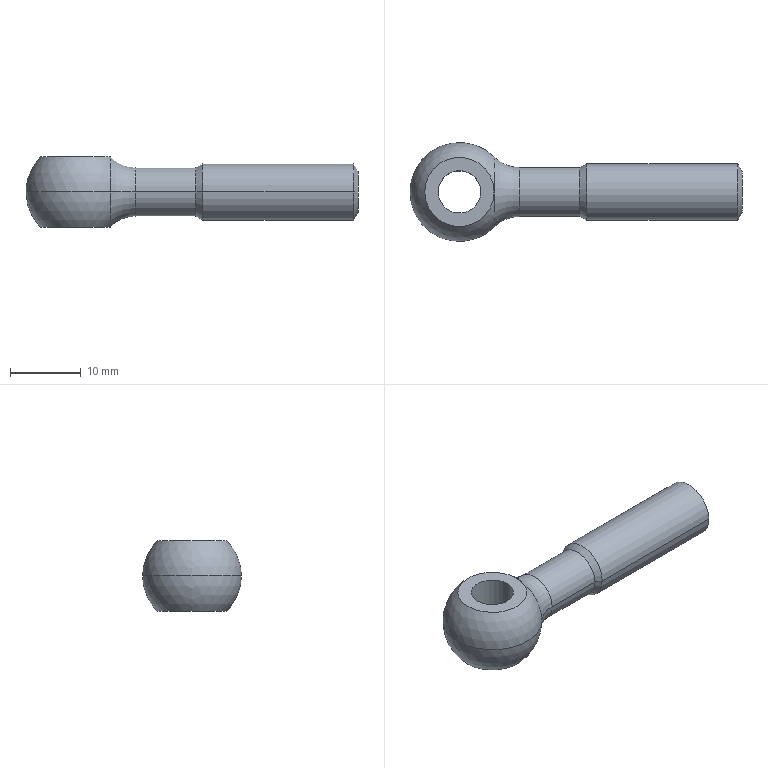Part | SolidWorks | features Cut 2, Revolution 2, Chamfer 1, Fillet 1, LPattern 1, RevCut 1 | 1 solid | 17 faces | box 47 x 14 x 10 mm | volume 2546 mm3 | cylinder 6 | cone 4 | plane 3 | torus 2 | sphere 2 | commonest cylinder face diameters 6 x2 6.918 x2 8 x2
STEP:
#1=CARTESIAN_POINT('',(4.965,4.934,0.));
#2=VERTEX_POINT('',#1);
#3=CARTESIAN_POINT('',(4.965,-4.934,0.));
#4=VERTEX_POINT('',#3);
#5=CARTESIAN_POINT('',(4.965,0.,0.));
#6=DIRECTION('',(-1.,0.,0.));
#7=DIRECTION('',(0.,-1.,0.));
#8=AXIS2_PLACEMENT_3D('',#5,#6,#7);
#9=CIRCLE('',#8,4.934);
#10=EDGE_CURVE('',#2,#4,#9,.T.);
#11=ORIENTED_EDGE('',*,*,#10,.F.);
#12=CARTESIAN_POINT('',(8.512,3.459,0.));
#13=VERTEX_POINT('',#12);
#14=CARTESIAN_POINT('',(8.512,8.459,0.));
#15=DIRECTION('',(0.,0.,1.));
#16=DIRECTION('',(0.,-1.,0.));
#17=AXIS2_PLACEMENT_3D('',#14,#15,#16);
#18=CIRCLE('',#17,5.);
#19=EDGE_CURVE('',#2,#13,#18,.T.);
#20=ORIENTED_EDGE('',*,*,#19,.T.);
#21=CARTESIAN_POINT('',(8.512,-3.459,0.));
#22=VERTEX_POINT('',#21);
#23=CARTESIAN_POINT('',(8.512,0.,0.));
#24=DIRECTION('',(1.,0.,0.));
#25=DIRECTION('',(0.,-1.,0.));
#26=AXIS2_PLACEMENT_3D('',#23,#24,#25);
#27=CIRCLE('',#26,3.459);
#28=EDGE_CURVE('',#22,#13,#27,.T.);
#29=ORIENTED_EDGE('',*,*,#28,.F.);
#30=CARTESIAN_POINT('',(8.512,-8.459,0.));
#31=DIRECTION('',(0.,0.,-1.));
#32=DIRECTION('',(0.,1.,0.));
#33=AXIS2_PLACEMENT_3D('',#30,#31,#32);
#34=CIRCLE('',#33,5.);
#35=EDGE_CURVE('',#4,#22,#34,.T.);
#36=ORIENTED_EDGE('',*,*,#35,.F.);
#37=EDGE_LOOP('',(#11,#20,#29,#36));
#38=FACE_OUTER_BOUND('',#37,.T.);
#39=CARTESIAN_POINT('',(8.512,0.,0.));
#40=DIRECTION('',(-1.,0.,0.));
#41=DIRECTION('',(0.,-1.,0.));
#42=AXIS2_PLACEMENT_3D('',#39,#40,#41);
#43=TOROIDAL_SURFACE('',#42,8.459,5.);
#44=ADVANCED_FACE('',(#38),#43,.F.);
#45=CARTESIAN_POINT('',(40.,-2.918,0.));
#46=VERTEX_POINT('',#45);
#47=CARTESIAN_POINT('',(40.,2.917,0.));
#48=VERTEX_POINT('',#47);
#49=CARTESIAN_POINT('',(40.,0.,0.));
#50=DIRECTION('',(-1.,0.,0.));
#51=DIRECTION('',(0.,-1.,0.));
#52=AXIS2_PLACEMENT_3D('',#49,#50,#51);
#53=CIRCLE('',#52,2.918);
#54=EDGE_CURVE('',#46,#48,#53,.T.);
#55=ORIENTED_EDGE('',*,*,#54,.T.);
#56=CARTESIAN_POINT('',(39.375,4.,0.));
#57=VERTEX_POINT('',#56);
#58=CARTESIAN_POINT('',(39.375,4.,0.));
#59=DIRECTION('',(-0.5,0.866,0.));
#60=VECTOR('',#59,1000.);
#61=LINE('',#58,#60);
#62=EDGE_CURVE('',#48,#57,#61,.T.);
#63=ORIENTED_EDGE('',*,*,#62,.T.);
#64=CARTESIAN_POINT('',(39.375,-4.,0.));
#65=VERTEX_POINT('',#64);
#66=CARTESIAN_POINT('',(39.375,0.,0.));
#67=DIRECTION('',(-1.,0.,0.));
#68=DIRECTION('',(0.,-1.,0.));
#69=AXIS2_PLACEMENT_3D('',#66,#67,#68);
#70=CIRCLE('',#69,4.);
#71=EDGE_CURVE('',#65,#57,#70,.T.);
#72=ORIENTED_EDGE('',*,*,#71,.F.);
#73=CARTESIAN_POINT('',(39.375,-4.,0.));
#74=DIRECTION('',(-0.5,-0.866,0.));
#75=VECTOR('',#74,1000.);
#76=LINE('',#73,#75);
#77=EDGE_CURVE('',#46,#65,#76,.T.);
#78=ORIENTED_EDGE('',*,*,#77,.F.);
#79=EDGE_LOOP('',(#55,#63,#72,#78));
#80=FACE_OUTER_BOUND('',#79,.T.);
#81=CARTESIAN_POINT('',(39.375,0.,0.));
#82=DIRECTION('',(-1.,0.,0.));
#83=DIRECTION('',(0.,-1.,0.));
#84=AXIS2_PLACEMENT_3D('',#81,#82,#83);
#85=CONICAL_SURFACE('',#84,4.,1.047);
#86=ADVANCED_FACE('',(#80),#85,.T.);
#87=CARTESIAN_POINT('',(17.063,-3.459,0.));
#88=VERTEX_POINT('',#87);
#89=CARTESIAN_POINT('',(17.063,3.459,0.));
#90=VERTEX_POINT('',#89);
#91=CARTESIAN_POINT('',(17.063,0.,0.));
#92=DIRECTION('',(-1.,0.,0.));
#93=DIRECTION('',(0.,-1.,0.));
#94=AXIS2_PLACEMENT_3D('',#91,#92,#93);
#95=CIRCLE('',#94,3.459);
#96=EDGE_CURVE('',#88,#90,#95,.T.);
#97=ORIENTED_EDGE('',*,*,#96,.F.);
#98=CARTESIAN_POINT('',(18.,-4.,0.));
#99=VERTEX_POINT('',#98);
#100=CARTESIAN_POINT('',(18.,-4.,0.));
#101=DIRECTION('',(0.866,-0.5,0.));
#102=VECTOR('',#101,1000.);
#103=LINE('',#100,#102);
#104=EDGE_CURVE('',#88,#99,#103,.T.);
#105=ORIENTED_EDGE('',*,*,#104,.T.);
#106=CARTESIAN_POINT('',(18.,4.,0.));
#107=VERTEX_POINT('',#106);
#108=CARTESIAN_POINT('',(18.,0.,0.));
#109=DIRECTION('',(-1.,0.,0.));
#110=DIRECTION('',(0.,-1.,0.));
#111=AXIS2_PLACEMENT_3D('',#108,#109,#110);
#112=CIRCLE('',#111,4.);
#113=EDGE_CURVE('',#99,#107,#112,.T.);
#114=ORIENTED_EDGE('',*,*,#113,.T.);
#115=CARTESIAN_POINT('',(18.,4.,0.));
#116=DIRECTION('',(0.866,0.5,0.));
#117=VECTOR('',#116,1000.);
#118=LINE('',#115,#117);
#119=EDGE_CURVE('',#90,#107,#118,.T.);
#120=ORIENTED_EDGE('',*,*,#119,.F.);
#121=EDGE_LOOP('',(#97,#105,#114,#120));
#122=FACE_OUTER_BOUND('',#121,.T.);
#123=CARTESIAN_POINT('',(18.,0.,0.));
#124=DIRECTION('',(1.,0.,0.));
#125=DIRECTION('',(0.,1.,0.));
#126=AXIS2_PLACEMENT_3D('',#123,#124,#125);
#127=CONICAL_SURFACE('',#126,4.,0.5236);
#128=ADVANCED_FACE('',(#122),#127,.T.);
#129=ORIENTED_EDGE('',*,*,#96,.T.);
#130=CARTESIAN_POINT('',(0.,3.459,0.));
#131=DIRECTION('',(-1.,0.,0.));
#132=VECTOR('',#131,1000.);
#133=LINE('',#130,#132);
#134=EDGE_CURVE('',#90,#13,#133,.T.);
#135=ORIENTED_EDGE('',*,*,#134,.T.);
#136=CARTESIAN_POINT('',(8.512,0.,0.));
#137=DIRECTION('',(1.,0.,0.));
#138=DIRECTION('',(0.,-1.,0.));
#139=AXIS2_PLACEMENT_3D('',#136,#137,#138);
#140=CIRCLE('',#139,3.459);
#141=EDGE_CURVE('',#13,#22,#140,.T.);
#142=ORIENTED_EDGE('',*,*,#141,.T.);
#143=CARTESIAN_POINT('',(0.,-3.459,0.));
#144=DIRECTION('',(-1.,0.,0.));
#145=VECTOR('',#144,1000.);
#146=LINE('',#143,#145);
#147=EDGE_CURVE('',#88,#22,#146,.T.);
#148=ORIENTED_EDGE('',*,*,#147,.F.);
#149=EDGE_LOOP('',(#129,#135,#142,#148));
#150=FACE_OUTER_BOUND('',#149,.T.);
#151=CARTESIAN_POINT('',(0.,0.,0.));
#152=DIRECTION('',(-1.,0.,0.));
#153=DIRECTION('',(0.,-1.,0.));
#154=AXIS2_PLACEMENT_3D('',#151,#152,#153);
#155=CYLINDRICAL_SURFACE('',#154,3.459);
#156=ADVANCED_FACE('',(#150),#155,.T.);
#157=CARTESIAN_POINT('',(-3.,0.,-5.));
#158=VERTEX_POINT('',#157);
#159=CARTESIAN_POINT('',(3.,0.,-5.));
#160=VERTEX_POINT('',#159);
#161=CARTESIAN_POINT('',(0.,0.,-5.));
#162=DIRECTION('',(0.,0.,1.));
#163=DIRECTION('',(1.,0.,0.));
#164=AXIS2_PLACEMENT_3D('',#161,#162,#163);
#165=CIRCLE('',#164,3.);
#166=EDGE_CURVE('',#158,#160,#165,.T.);
#167=ORIENTED_EDGE('',*,*,#166,.F.);
#168=CARTESIAN_POINT('',(-3.,0.,5.));
#169=VERTEX_POINT('',#168);
#170=CARTESIAN_POINT('',(-3.,0.,-5.));
#171=DIRECTION('',(0.,0.,1.));
#172=VECTOR('',#171,1000.);
#173=LINE('',#170,#172);
#174=EDGE_CURVE('',#158,#169,#173,.T.);
#175=ORIENTED_EDGE('',*,*,#174,.T.);
#176=CARTESIAN_POINT('',(3.,0.,5.));
#177=VERTEX_POINT('',#176);
#178=CARTESIAN_POINT('',(0.,0.,5.));
#179=DIRECTION('',(0.,0.,1.));
#180=DIRECTION('',(1.,0.,0.));
#181=AXIS2_PLACEMENT_3D('',#178,#179,#180);
#182=CIRCLE('',#181,3.);
#183=EDGE_CURVE('',#169,#177,#182,.T.);
#184=ORIENTED_EDGE('',*,*,#183,.T.);
#185=CARTESIAN_POINT('',(3.,0.,-5.));
#186=DIRECTION('',(0.,0.,1.));
#187=VECTOR('',#186,1000.);
#188=LINE('',#185,#187);
#189=EDGE_CURVE('',#160,#177,#188,.T.);
#190=ORIENTED_EDGE('',*,*,#189,.F.);
#191=EDGE_LOOP('',(#167,#175,#184,#190));
#192=FACE_OUTER_BOUND('',#191,.T.);
#193=CARTESIAN_POINT('',(0.,0.,-5.));
#194=DIRECTION('',(0.,0.,1.));
#195=DIRECTION('',(1.,0.,0.));
#196=AXIS2_PLACEMENT_3D('',#193,#194,#195);
#197=CYLINDRICAL_SURFACE('',#196,3.);
#198=ADVANCED_FACE('',(#192),#197,.F.);
#199=CARTESIAN_POINT('',(4.899,0.,-5.));
#200=VERTEX_POINT('',#199);
#201=CARTESIAN_POINT('',(-4.899,0.,-5.));
#202=VERTEX_POINT('',#201);
#203=CARTESIAN_POINT('',(0.,0.,-5.));
#204=DIRECTION('',(0.,0.,1.));
#205=DIRECTION('',(1.,0.,0.));
#206=AXIS2_PLACEMENT_3D('',#203,#204,#205);
#207=CIRCLE('',#206,4.899);
#208=EDGE_CURVE('',#200,#202,#207,.T.);
#209=ORIENTED_EDGE('',*,*,#208,.T.);
#210=CARTESIAN_POINT('',(0.,0.,-5.));
#211=DIRECTION('',(0.,0.,1.));
#212=DIRECTION('',(1.,0.,0.));
#213=AXIS2_PLACEMENT_3D('',#210,#211,#212);
#214=CIRCLE('',#213,4.899);
#215=EDGE_CURVE('',#202,#200,#214,.T.);
#216=ORIENTED_EDGE('',*,*,#215,.T.);
#217=EDGE_LOOP('',(#209,#216));
#218=FACE_BOUND('',#217,.T.);
#219=ORIENTED_EDGE('',*,*,#10,.T.);
#220=CARTESIAN_POINT('',(-7.,0.,0.));
#221=VERTEX_POINT('',#220);
#222=CARTESIAN_POINT('',(0.,0.,0.));
#223=DIRECTION('',(0.,0.,-1.));
#224=DIRECTION('',(0.,1.,0.));
#225=AXIS2_PLACEMENT_3D('',#222,#223,#224);
#226=CIRCLE('',#225,7.);
#227=EDGE_CURVE('',#4,#221,#226,.T.);
#228=ORIENTED_EDGE('',*,*,#227,.T.);
#229=CARTESIAN_POINT('',(0.,0.,0.));
#230=DIRECTION('',(0.,0.,1.));
#231=DIRECTION('',(0.,-1.,0.));
#232=AXIS2_PLACEMENT_3D('',#229,#230,#231);
#233=CIRCLE('',#232,7.);
#234=EDGE_CURVE('',#2,#221,#233,.T.);
#235=ORIENTED_EDGE('',*,*,#234,.F.);
#236=EDGE_LOOP('',(#219,#228,#235));
#237=FACE_OUTER_BOUND('',#236,.T.);
#238=CARTESIAN_POINT('',(0.,0.,0.));
#239=DIRECTION('',(0.,0.,-1.));
#240=DIRECTION('',(0.,1.,0.));
#241=AXIS2_PLACEMENT_3D('',#238,#239,#240);
#242=SPHERICAL_SURFACE('',#241,7.);
#243=ADVANCED_FACE('',(#218,#237),#242,.T.);
#244=ORIENTED_EDGE('',*,*,#71,.T.);
#245=CARTESIAN_POINT('',(0.,4.,0.));
#246=DIRECTION('',(-1.,0.,0.));
#247=VECTOR('',#246,1000.);
#248=LINE('',#245,#247);
#249=EDGE_CURVE('',#57,#107,#248,.T.);
#250=ORIENTED_EDGE('',*,*,#249,.T.);
#251=ORIENTED_EDGE('',*,*,#113,.F.);
#252=CARTESIAN_POINT('',(0.,-4.,0.));
#253=DIRECTION('',(-1.,0.,0.));
#254=VECTOR('',#253,1000.);
#255=LINE('',#252,#254);
#256=EDGE_CURVE('',#65,#99,#255,.T.);
#257=ORIENTED_EDGE('',*,*,#256,.F.);
#258=EDGE_LOOP('',(#244,#250,#251,#257));
#259=FACE_OUTER_BOUND('',#258,.T.);
#260=CARTESIAN_POINT('',(0.,0.,0.));
#261=DIRECTION('',(-1.,0.,0.));
#262=DIRECTION('',(0.,-1.,0.));
#263=AXIS2_PLACEMENT_3D('',#260,#261,#262);
#264=CYLINDRICAL_SURFACE('',#263,4.);
#265=ADVANCED_FACE('',(#259),#264,.T.);
#266=ORIENTED_EDGE('',*,*,#249,.F.);
#267=CARTESIAN_POINT('',(39.375,0.,0.));
#268=DIRECTION('',(-1.,0.,0.));
#269=DIRECTION('',(0.,-1.,0.));
#270=AXIS2_PLACEMENT_3D('',#267,#268,#269);
#271=CIRCLE('',#270,4.);
#272=EDGE_CURVE('',#57,#65,#271,.T.);
#273=ORIENTED_EDGE('',*,*,#272,.T.);
#274=ORIENTED_EDGE('',*,*,#256,.T.);
#275=CARTESIAN_POINT('',(18.,0.,0.));
#276=DIRECTION('',(-1.,0.,0.));
#277=DIRECTION('',(0.,-1.,0.));
#278=AXIS2_PLACEMENT_3D('',#275,#276,#277);
#279=CIRCLE('',#278,4.);
#280=EDGE_CURVE('',#107,#99,#279,.T.);
#281=ORIENTED_EDGE('',*,*,#280,.F.);
#282=EDGE_LOOP('',(#266,#273,#274,#281));
#283=FACE_OUTER_BOUND('',#282,.T.);
#284=CARTESIAN_POINT('',(0.,0.,0.));
#285=DIRECTION('',(-1.,0.,0.));
#286=DIRECTION('',(0.,-1.,0.));
#287=AXIS2_PLACEMENT_3D('',#284,#285,#286);
#288=CYLINDRICAL_SURFACE('',#287,4.);
#289=ADVANCED_FACE('',(#283),#288,.T.);
#290=ORIENTED_EDGE('',*,*,#227,.F.);
#291=CARTESIAN_POINT('',(4.965,0.,0.));
#292=DIRECTION('',(-1.,0.,0.));
#293=DIRECTION('',(0.,-1.,0.));
#294=AXIS2_PLACEMENT_3D('',#291,#292,#293);
#295=CIRCLE('',#294,4.934);
#296=EDGE_CURVE('',#4,#2,#295,.T.);
#297=ORIENTED_EDGE('',*,*,#296,.T.);
#298=ORIENTED_EDGE('',*,*,#234,.T.);
#299=EDGE_LOOP('',(#290,#297,#298));
#300=FACE_OUTER_BOUND('',#299,.T.);
#301=CARTESIAN_POINT('',(-4.899,0.,5.));
#302=VERTEX_POINT('',#301);
#303=CARTESIAN_POINT('',(4.899,0.,5.));
#304=VERTEX_POINT('',#303);
#305=CARTESIAN_POINT('',(0.,0.,5.));
#306=DIRECTION('',(0.,0.,-1.));
#307=DIRECTION('',(-1.,0.,0.));
#308=AXIS2_PLACEMENT_3D('',#305,#306,#307);
#309=CIRCLE('',#308,4.899);
#310=EDGE_CURVE('',#302,#304,#309,.T.);
#311=ORIENTED_EDGE('',*,*,#310,.T.);
#312=CARTESIAN_POINT('',(0.,0.,5.));
#313=DIRECTION('',(0.,0.,-1.));
#314=DIRECTION('',(-1.,0.,0.));
#315=AXIS2_PLACEMENT_3D('',#312,#313,#314);
#316=CIRCLE('',#315,4.899);
#317=EDGE_CURVE('',#304,#302,#316,.T.);
#318=ORIENTED_EDGE('',*,*,#317,.T.);
#319=EDGE_LOOP('',(#311,#318));
#320=FACE_BOUND('',#319,.T.);
#321=CARTESIAN_POINT('',(0.,0.,0.));
#322=DIRECTION('',(0.,0.,-1.));
#323=DIRECTION('',(0.,1.,0.));
#324=AXIS2_PLACEMENT_3D('',#321,#322,#323);
#325=SPHERICAL_SURFACE('',#324,7.);
#326=ADVANCED_FACE('',(#300,#320),#325,.T.);
#327=CARTESIAN_POINT('',(0.,0.,5.));
#328=DIRECTION('',(0.,0.,1.));
#329=DIRECTION('',(1.,0.,0.));
#330=AXIS2_PLACEMENT_3D('',#327,#328,#329);
#331=CIRCLE('',#330,3.);
#332=EDGE_CURVE('',#177,#169,#331,.T.);
#333=ORIENTED_EDGE('',*,*,#332,.F.);
#334=ORIENTED_EDGE('',*,*,#183,.F.);
#335=EDGE_LOOP('',(#333,#334));
#336=FACE_BOUND('',#335,.T.);
#337=ORIENTED_EDGE('',*,*,#310,.F.);
#338=ORIENTED_EDGE('',*,*,#317,.F.);
#339=EDGE_LOOP('',(#337,#338));
#340=FACE_OUTER_BOUND('',#339,.T.);
#341=CARTESIAN_POINT('',(-7.,4.899,5.));
#342=DIRECTION('',(0.,0.,-1.));
#343=DIRECTION('',(-1.,0.,0.));
#344=AXIS2_PLACEMENT_3D('',#341,#342,#343);
#345=PLANE('',#344);
#346=ADVANCED_FACE('',(#336,#340),#345,.F.);
#347=CARTESIAN_POINT('',(0.,0.,-5.));
#348=DIRECTION('',(0.,0.,1.));
#349=DIRECTION('',(1.,0.,0.));
#350=AXIS2_PLACEMENT_3D('',#347,#348,#349);
#351=CIRCLE('',#350,3.);
#352=EDGE_CURVE('',#160,#158,#351,.T.);
#353=ORIENTED_EDGE('',*,*,#352,.T.);
#354=ORIENTED_EDGE('',*,*,#166,.T.);
#355=EDGE_LOOP('',(#353,#354));
#356=FACE_BOUND('',#355,.T.);
#357=ORIENTED_EDGE('',*,*,#208,.F.);
#358=ORIENTED_EDGE('',*,*,#215,.F.);
#359=EDGE_LOOP('',(#357,#358));
#360=FACE_OUTER_BOUND('',#359,.T.);
#361=CARTESIAN_POINT('',(-7.,4.899,-5.));
#362=DIRECTION('',(0.,0.,1.));
#363=DIRECTION('',(1.,0.,0.));
#364=AXIS2_PLACEMENT_3D('',#361,#362,#363);
#365=PLANE('',#364);
#366=ADVANCED_FACE('',(#356,#360),#365,.F.);
#367=ORIENTED_EDGE('',*,*,#174,.F.);
#368=ORIENTED_EDGE('',*,*,#352,.F.);
#369=ORIENTED_EDGE('',*,*,#189,.T.);
#370=ORIENTED_EDGE('',*,*,#332,.T.);
#371=EDGE_LOOP('',(#367,#368,#369,#370));
#372=FACE_OUTER_BOUND('',#371,.T.);
#373=CARTESIAN_POINT('',(0.,0.,-5.));
#374=DIRECTION('',(0.,0.,1.));
#375=DIRECTION('',(1.,0.,0.));
#376=AXIS2_PLACEMENT_3D('',#373,#374,#375);
#377=CYLINDRICAL_SURFACE('',#376,3.);
#378=ADVANCED_FACE('',(#372),#377,.F.);
#379=ORIENTED_EDGE('',*,*,#134,.F.);
#380=CARTESIAN_POINT('',(17.063,0.,0.));
#381=DIRECTION('',(-1.,0.,0.));
#382=DIRECTION('',(0.,-1.,0.));
#383=AXIS2_PLACEMENT_3D('',#380,#381,#382);
#384=CIRCLE('',#383,3.459);
#385=EDGE_CURVE('',#90,#88,#384,.T.);
#386=ORIENTED_EDGE('',*,*,#385,.T.);
#387=ORIENTED_EDGE('',*,*,#147,.T.);
#388=ORIENTED_EDGE('',*,*,#28,.T.);
#389=EDGE_LOOP('',(#379,#386,#387,#388));
#390=FACE_OUTER_BOUND('',#389,.T.);
#391=CARTESIAN_POINT('',(0.,0.,0.));
#392=DIRECTION('',(-1.,0.,0.));
#393=DIRECTION('',(0.,-1.,0.));
#394=AXIS2_PLACEMENT_3D('',#391,#392,#393);
#395=CYLINDRICAL_SURFACE('',#394,3.459);
#396=ADVANCED_FACE('',(#390),#395,.T.);
#397=ORIENTED_EDGE('',*,*,#104,.F.);
#398=ORIENTED_EDGE('',*,*,#385,.F.);
#399=ORIENTED_EDGE('',*,*,#119,.T.);
#400=ORIENTED_EDGE('',*,*,#280,.T.);
#401=EDGE_LOOP('',(#397,#398,#399,#400));
#402=FACE_OUTER_BOUND('',#401,.T.);
#403=CARTESIAN_POINT('',(18.,0.,0.));
#404=DIRECTION('',(1.,0.,0.));
#405=DIRECTION('',(0.,1.,0.));
#406=AXIS2_PLACEMENT_3D('',#403,#404,#405);
#407=CONICAL_SURFACE('',#406,4.,0.5236);
#408=ADVANCED_FACE('',(#402),#407,.T.);
#409=ORIENTED_EDGE('',*,*,#62,.F.);
#410=CARTESIAN_POINT('',(40.,0.,0.));
#411=DIRECTION('',(-1.,0.,0.));
#412=DIRECTION('',(0.,-1.,0.));
#413=AXIS2_PLACEMENT_3D('',#410,#411,#412);
#414=CIRCLE('',#413,2.918);
#415=EDGE_CURVE('',#48,#46,#414,.T.);
#416=ORIENTED_EDGE('',*,*,#415,.T.);
#417=ORIENTED_EDGE('',*,*,#77,.T.);
#418=ORIENTED_EDGE('',*,*,#272,.F.);
#419=EDGE_LOOP('',(#409,#416,#417,#418));
#420=FACE_OUTER_BOUND('',#419,.T.);
#421=CARTESIAN_POINT('',(39.375,0.,0.));
#422=DIRECTION('',(-1.,0.,0.));
#423=DIRECTION('',(0.,-1.,0.));
#424=AXIS2_PLACEMENT_3D('',#421,#422,#423);
#425=CONICAL_SURFACE('',#424,4.,1.047);
#426=ADVANCED_FACE('',(#420),#425,.T.);
#427=ORIENTED_EDGE('',*,*,#54,.F.);
#428=ORIENTED_EDGE('',*,*,#415,.F.);
#429=EDGE_LOOP('',(#427,#428));
#430=FACE_OUTER_BOUND('',#429,.T.);
#431=CARTESIAN_POINT('',(40.,4.,0.));
#432=DIRECTION('',(-1.,0.,0.));
#433=DIRECTION('',(0.,-1.,0.));
#434=AXIS2_PLACEMENT_3D('',#431,#432,#433);
#435=PLANE('',#434);
#436=ADVANCED_FACE('',(#430),#435,.F.);
#437=ORIENTED_EDGE('',*,*,#19,.F.);
#438=ORIENTED_EDGE('',*,*,#296,.F.);
#439=ORIENTED_EDGE('',*,*,#35,.T.);
#440=ORIENTED_EDGE('',*,*,#141,.F.);
#441=EDGE_LOOP('',(#437,#438,#439,#440));
#442=FACE_OUTER_BOUND('',#441,.T.);
#443=CARTESIAN_POINT('',(8.512,0.,0.));
#444=DIRECTION('',(-1.,0.,0.));
#445=DIRECTION('',(0.,-1.,0.));
#446=AXIS2_PLACEMENT_3D('',#443,#444,#445);
#447=TOROIDAL_SURFACE('',#446,8.459,5.);
#448=ADVANCED_FACE('',(#442),#447,.F.);
#449=CLOSED_SHELL('',(#44,#86,#128,#156,#198,#243,#265,#289,#326,#346,#366,#378,#396,#408,#426,#436,#448));
#450=MANIFOLD_SOLID_BREP('',#449);
#451=CARTESIAN_POINT('',(0.,0.,0.));
#452=DIRECTION('',(0.,0.,1.));
#453=DIRECTION('',(1.,0.,0.));
#454=AXIS2_PLACEMENT_3D('',#451,#452,#453);
#455=(LENGTH_UNIT()NAMED_UNIT(*)SI_UNIT(.MILLI.,.METRE.));
#456=UNCERTAINTY_MEASURE_WITH_UNIT(LENGTH_MEASURE(0.00001),#455,'','');
#457=(NAMED_UNIT(*)PLANE_ANGLE_UNIT()SI_UNIT($,.RADIAN.));
#458=(NAMED_UNIT(*)SI_UNIT($,.STERADIAN.)SOLID_ANGLE_UNIT());
#459=(GEOMETRIC_REPRESENTATION_CONTEXT(3)GLOBAL_UNCERTAINTY_ASSIGNED_CONTEXT((#456))GLOBAL_UNIT_ASSIGNED_CONTEXT((#455,#457,#458))REPRESENTATION_CONTEXT('',''));
#460=ADVANCED_BREP_SHAPE_REPRESENTATION('',(#450,#454),#459);